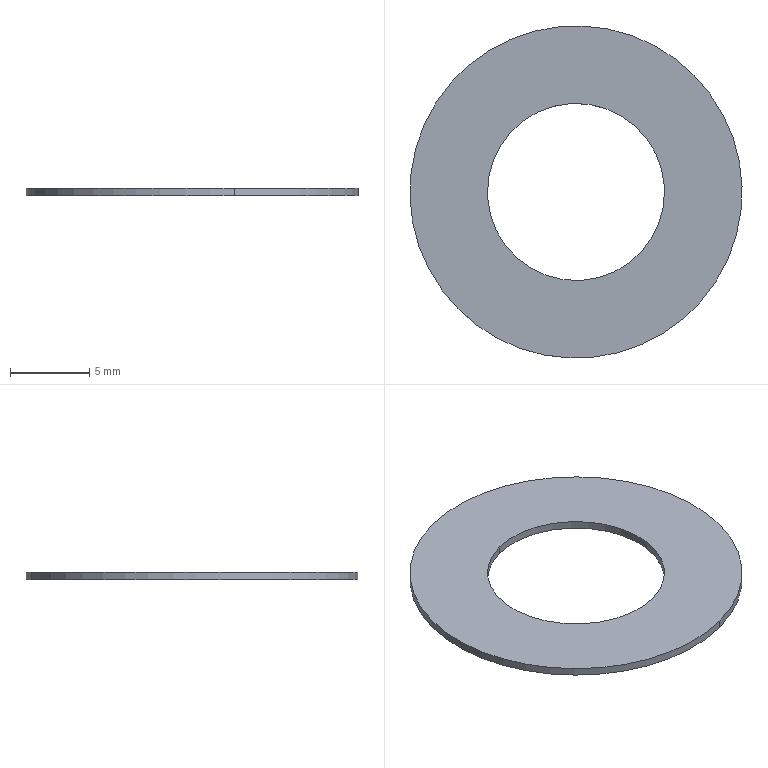Part | SolidWorks | features BaseBody 1 | 1 solid | 6 faces | box 21 x 21 x 0.5 mm | volume 123.92 mm3 | cylinder 4 | plane 2 | commonest cylinder face diameters 11.2 x2 21 x2
STEP:
#1=CARTESIAN_POINT('',(384.522,97.084,50.));
#2=VERTEX_POINT('',#1);
#3=CARTESIAN_POINT('',(381.678,107.916,50.));
#4=VERTEX_POINT('',#3);
#5=CARTESIAN_POINT('',(383.1,102.5,50.));
#6=DIRECTION('',(0.,0.,1.));
#7=DIRECTION('',(-0.254,0.9672,0.));
#8=AXIS2_PLACEMENT_3D('',#5,#6,#7);
#9=CIRCLE('',#8,5.6);
#10=EDGE_CURVE('',#2,#4,#9,.T.);
#11=ORIENTED_EDGE('',*,*,#10,.T.);
#12=CARTESIAN_POINT('',(381.678,107.916,49.5));
#13=VERTEX_POINT('',#12);
#14=CARTESIAN_POINT('',(381.678,107.916,50.));
#15=DIRECTION('',(0.,0.,-1.));
#16=VECTOR('',#15,1000.);
#17=LINE('',#14,#16);
#18=EDGE_CURVE('',#4,#13,#17,.T.);
#19=ORIENTED_EDGE('',*,*,#18,.T.);
#20=CARTESIAN_POINT('',(384.522,97.084,49.5));
#21=VERTEX_POINT('',#20);
#22=CARTESIAN_POINT('',(383.1,102.5,49.5));
#23=DIRECTION('',(0.,0.,1.));
#24=DIRECTION('',(-0.254,0.9672,0.));
#25=AXIS2_PLACEMENT_3D('',#22,#23,#24);
#26=CIRCLE('',#25,5.6);
#27=EDGE_CURVE('',#21,#13,#26,.T.);
#28=ORIENTED_EDGE('',*,*,#27,.F.);
#29=CARTESIAN_POINT('',(384.522,97.084,50.));
#30=DIRECTION('',(0.,0.,-1.));
#31=VECTOR('',#30,1000.);
#32=LINE('',#29,#31);
#33=EDGE_CURVE('',#2,#21,#32,.T.);
#34=ORIENTED_EDGE('',*,*,#33,.F.);
#35=EDGE_LOOP('',(#11,#19,#28,#34));
#36=FACE_OUTER_BOUND('',#35,.T.);
#37=CARTESIAN_POINT('',(383.1,102.5,50.));
#38=DIRECTION('',(0.,0.,-1.));
#39=DIRECTION('',(0.254,-0.9672,0.));
#40=AXIS2_PLACEMENT_3D('',#37,#38,#39);
#41=CYLINDRICAL_SURFACE('',#40,5.6);
#42=ADVANCED_FACE('',(#36),#41,.F.);
#43=CARTESIAN_POINT('',(380.433,112.656,50.));
#44=VERTEX_POINT('',#43);
#45=CARTESIAN_POINT('',(385.767,92.344,50.));
#46=VERTEX_POINT('',#45);
#47=CARTESIAN_POINT('',(383.1,102.5,50.));
#48=DIRECTION('',(0.,0.,1.));
#49=DIRECTION('',(-0.254,0.9672,0.));
#50=AXIS2_PLACEMENT_3D('',#47,#48,#49);
#51=CIRCLE('',#50,10.5);
#52=EDGE_CURVE('',#44,#46,#51,.T.);
#53=ORIENTED_EDGE('',*,*,#52,.F.);
#54=CARTESIAN_POINT('',(380.433,112.656,49.5));
#55=VERTEX_POINT('',#54);
#56=CARTESIAN_POINT('',(380.433,112.656,50.));
#57=DIRECTION('',(0.,0.,-1.));
#58=VECTOR('',#57,1000.);
#59=LINE('',#56,#58);
#60=EDGE_CURVE('',#44,#55,#59,.T.);
#61=ORIENTED_EDGE('',*,*,#60,.T.);
#62=CARTESIAN_POINT('',(385.767,92.344,49.5));
#63=VERTEX_POINT('',#62);
#64=CARTESIAN_POINT('',(383.1,102.5,49.5));
#65=DIRECTION('',(0.,0.,1.));
#66=DIRECTION('',(-0.254,0.9672,0.));
#67=AXIS2_PLACEMENT_3D('',#64,#65,#66);
#68=CIRCLE('',#67,10.5);
#69=EDGE_CURVE('',#55,#63,#68,.T.);
#70=ORIENTED_EDGE('',*,*,#69,.T.);
#71=CARTESIAN_POINT('',(385.767,92.344,50.));
#72=DIRECTION('',(0.,0.,-1.));
#73=VECTOR('',#72,1000.);
#74=LINE('',#71,#73);
#75=EDGE_CURVE('',#46,#63,#74,.T.);
#76=ORIENTED_EDGE('',*,*,#75,.F.);
#77=EDGE_LOOP('',(#53,#61,#70,#76));
#78=FACE_OUTER_BOUND('',#77,.T.);
#79=CARTESIAN_POINT('',(383.1,102.5,50.));
#80=DIRECTION('',(0.,0.,-1.));
#81=DIRECTION('',(0.254,-0.9672,0.));
#82=AXIS2_PLACEMENT_3D('',#79,#80,#81);
#83=CYLINDRICAL_SURFACE('',#82,10.5);
#84=ADVANCED_FACE('',(#78),#83,.T.);
#85=CARTESIAN_POINT('',(383.1,102.5,50.));
#86=DIRECTION('',(0.,0.,1.));
#87=DIRECTION('',(-0.254,0.9672,0.));
#88=AXIS2_PLACEMENT_3D('',#85,#86,#87);
#89=CIRCLE('',#88,10.5);
#90=EDGE_CURVE('',#46,#44,#89,.T.);
#91=ORIENTED_EDGE('',*,*,#90,.T.);
#92=ORIENTED_EDGE('',*,*,#52,.T.);
#93=EDGE_LOOP('',(#91,#92));
#94=FACE_OUTER_BOUND('',#93,.T.);
#95=ORIENTED_EDGE('',*,*,#10,.F.);
#96=CARTESIAN_POINT('',(383.1,102.5,50.));
#97=DIRECTION('',(0.,0.,1.));
#98=DIRECTION('',(-0.254,0.9672,0.));
#99=AXIS2_PLACEMENT_3D('',#96,#97,#98);
#100=CIRCLE('',#99,5.6);
#101=EDGE_CURVE('',#4,#2,#100,.T.);
#102=ORIENTED_EDGE('',*,*,#101,.F.);
#103=EDGE_LOOP('',(#95,#102));
#104=FACE_BOUND('',#103,.T.);
#105=CARTESIAN_POINT('',(383.1,102.5,50.));
#106=DIRECTION('',(0.,0.,1.));
#107=DIRECTION('',(-0.254,0.9672,0.));
#108=AXIS2_PLACEMENT_3D('',#105,#106,#107);
#109=PLANE('',#108);
#110=ADVANCED_FACE('',(#94,#104),#109,.T.);
#111=CARTESIAN_POINT('',(383.1,102.5,49.5));
#112=DIRECTION('',(0.,0.,1.));
#113=DIRECTION('',(-0.254,0.9672,0.));
#114=AXIS2_PLACEMENT_3D('',#111,#112,#113);
#115=CIRCLE('',#114,10.5);
#116=EDGE_CURVE('',#63,#55,#115,.T.);
#117=ORIENTED_EDGE('',*,*,#116,.F.);
#118=ORIENTED_EDGE('',*,*,#69,.F.);
#119=EDGE_LOOP('',(#117,#118));
#120=FACE_OUTER_BOUND('',#119,.T.);
#121=ORIENTED_EDGE('',*,*,#27,.T.);
#122=CARTESIAN_POINT('',(383.1,102.5,49.5));
#123=DIRECTION('',(0.,0.,1.));
#124=DIRECTION('',(-0.254,0.9672,0.));
#125=AXIS2_PLACEMENT_3D('',#122,#123,#124);
#126=CIRCLE('',#125,5.6);
#127=EDGE_CURVE('',#13,#21,#126,.T.);
#128=ORIENTED_EDGE('',*,*,#127,.T.);
#129=EDGE_LOOP('',(#121,#128));
#130=FACE_BOUND('',#129,.T.);
#131=CARTESIAN_POINT('',(383.1,102.5,49.5));
#132=DIRECTION('',(0.,0.,1.));
#133=DIRECTION('',(-0.254,0.9672,0.));
#134=AXIS2_PLACEMENT_3D('',#131,#132,#133);
#135=PLANE('',#134);
#136=ADVANCED_FACE('',(#120,#130),#135,.F.);
#137=ORIENTED_EDGE('',*,*,#60,.F.);
#138=ORIENTED_EDGE('',*,*,#90,.F.);
#139=ORIENTED_EDGE('',*,*,#75,.T.);
#140=ORIENTED_EDGE('',*,*,#116,.T.);
#141=EDGE_LOOP('',(#137,#138,#139,#140));
#142=FACE_OUTER_BOUND('',#141,.T.);
#143=CARTESIAN_POINT('',(383.1,102.5,50.));
#144=DIRECTION('',(0.,0.,-1.));
#145=DIRECTION('',(0.254,-0.9672,0.));
#146=AXIS2_PLACEMENT_3D('',#143,#144,#145);
#147=CYLINDRICAL_SURFACE('',#146,10.5);
#148=ADVANCED_FACE('',(#142),#147,.T.);
#149=ORIENTED_EDGE('',*,*,#18,.F.);
#150=ORIENTED_EDGE('',*,*,#101,.T.);
#151=ORIENTED_EDGE('',*,*,#33,.T.);
#152=ORIENTED_EDGE('',*,*,#127,.F.);
#153=EDGE_LOOP('',(#149,#150,#151,#152));
#154=FACE_OUTER_BOUND('',#153,.T.);
#155=CARTESIAN_POINT('',(383.1,102.5,50.));
#156=DIRECTION('',(0.,0.,-1.));
#157=DIRECTION('',(0.254,-0.9672,0.));
#158=AXIS2_PLACEMENT_3D('',#155,#156,#157);
#159=CYLINDRICAL_SURFACE('',#158,5.6);
#160=ADVANCED_FACE('',(#154),#159,.F.);
#161=CLOSED_SHELL('',(#42,#84,#110,#136,#148,#160));
#162=MANIFOLD_SOLID_BREP('',#161);
#163=CARTESIAN_POINT('',(0.,0.,0.));
#164=DIRECTION('',(0.,0.,1.));
#165=DIRECTION('',(1.,0.,0.));
#166=AXIS2_PLACEMENT_3D('',#163,#164,#165);
#167=(LENGTH_UNIT()NAMED_UNIT(*)SI_UNIT(.MILLI.,.METRE.));
#168=UNCERTAINTY_MEASURE_WITH_UNIT(LENGTH_MEASURE(0.00001),#167,'','');
#169=(NAMED_UNIT(*)PLANE_ANGLE_UNIT()SI_UNIT($,.RADIAN.));
#170=(NAMED_UNIT(*)SI_UNIT($,.STERADIAN.)SOLID_ANGLE_UNIT());
#171=(GEOMETRIC_REPRESENTATION_CONTEXT(3)GLOBAL_UNCERTAINTY_ASSIGNED_CONTEXT((#168))GLOBAL_UNIT_ASSIGNED_CONTEXT((#167,#169,#170))REPRESENTATION_CONTEXT('',''));
#172=ADVANCED_BREP_SHAPE_REPRESENTATION('',(#162,#166),#171);